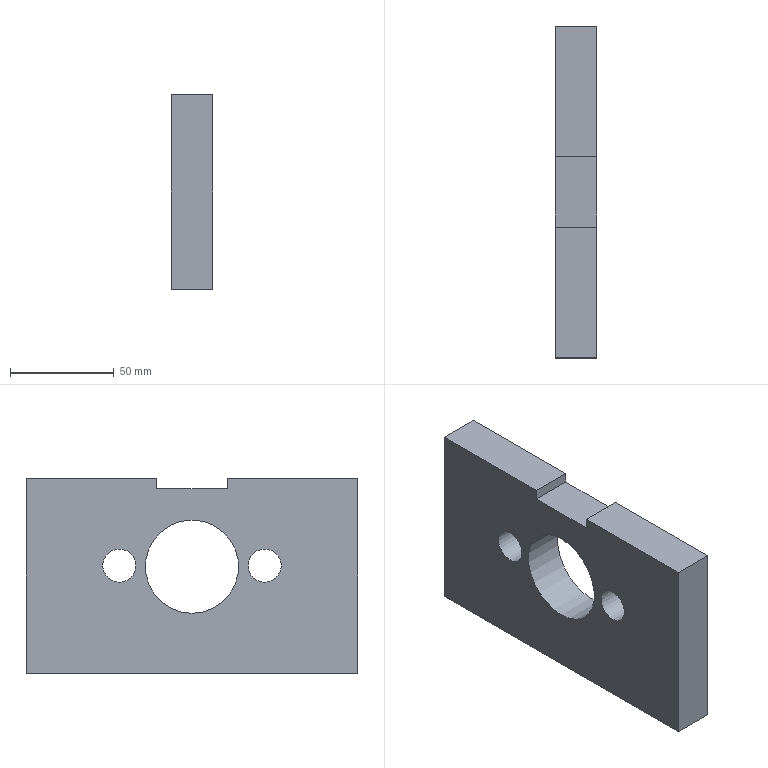Part | STEP file | Tube feed_id382_x_t | 1 solid | 13 faces | box 20 x 160 x 94 mm | volume 257549 mm3 | plane 10 | cylinder 3 | commonest cylinder face diameters 16 x2 45 x1
STEP:
#1=CARTESIAN_POINT('',(0.,0.,0.));
#2=DIRECTION('',(0.,0.,1.));
#3=DIRECTION('',(1.,0.,0.));
#4=AXIS2_PLACEMENT_3D('',#1,#2,#3);
#5=CARTESIAN_POINT('',(466.,446.936,-51.));
#6=VERTEX_POINT('',#5);
#7=CARTESIAN_POINT('',(466.,446.936,-43.));
#8=DIRECTION('',(-1.,0.,0.));
#9=DIRECTION('',(0.,0.,-1.));
#10=AXIS2_PLACEMENT_3D('',#7,#8,#9);
#11=CIRCLE('',#10,8.);
#12=CARTESIAN_POINT('',(466.,0.,0.));
#13=DIRECTION('',(1.,0.,0.));
#14=DIRECTION('',(0.,0.,-1.));
#15=AXIS2_PLACEMENT_3D('',#12,#13,#14);
#16=PLANE('',#15);
#17=CARTESIAN_POINT('',(51.,446.936));
#18=CARTESIAN_POINT('',(51.,433.079));
#19=CARTESIAN_POINT('',(39.,440.007));
#20=CARTESIAN_POINT('',(27.,446.936));
#21=CARTESIAN_POINT('',(39.,453.864));
#22=CARTESIAN_POINT('',(51.,460.792));
#23=CARTESIAN_POINT('',(51.,446.936));
#24=(BOUNDED_CURVE()B_SPLINE_CURVE(2,(#17,#18,#19,#20,#21,#22,#23),.UNSPECIFIED.,.T.,.F.)B_SPLINE_CURVE_WITH_KNOTS((1,2,2,2,2,1),(-2.094,0.,2.094,4.189,6.283,8.378),.UNSPECIFIED.)CURVE()GEOMETRIC_REPRESENTATION_ITEM()RATIONAL_B_SPLINE_CURVE((1.,0.5,1.,0.5,1.,0.5,1.))REPRESENTATION_ITEM(''));
#25=(GEOMETRIC_REPRESENTATION_CONTEXT(2)PARAMETRIC_REPRESENTATION_CONTEXT()REPRESENTATION_CONTEXT('',''));
#26=DEFINITIONAL_REPRESENTATION('',(#24),#25);
#27=PCURVE('',#16,#26);
#28=CARTESIAN_POINT('',(466.,446.936,-43.));
#29=DIRECTION('',(-1.,0.,0.));
#30=DIRECTION('',(0.,0.,1.));
#31=AXIS2_PLACEMENT_3D('',#28,#29,#30);
#32=CYLINDRICAL_SURFACE('',#31,8.);
#33=CARTESIAN_POINT('',(3.142,0.));
#34=DIRECTION('',(1.,0.));
#35=VECTOR('',#34,1.);
#36=LINE('',#33,#35);
#37=(GEOMETRIC_REPRESENTATION_CONTEXT(2)PARAMETRIC_REPRESENTATION_CONTEXT()REPRESENTATION_CONTEXT('',''));
#38=DEFINITIONAL_REPRESENTATION('',(#36),#37);
#39=PCURVE('',#32,#38);
#40=SURFACE_CURVE('',#11,(#27,#39),.PCURVE_S1.);
#41=EDGE_CURVE('',#6,#6,#40,.T.);
#42=ORIENTED_EDGE('',*,*,#41,.T.);
#43=EDGE_LOOP('',(#42));
#44=FACE_BOUND('',#43,.T.);
#45=CARTESIAN_POINT('',(466.,411.936,-66.));
#46=VERTEX_POINT('',#45);
#47=CARTESIAN_POINT('',(466.,411.936,-43.5));
#48=DIRECTION('',(-1.,0.,0.));
#49=DIRECTION('',(0.,0.,-1.));
#50=AXIS2_PLACEMENT_3D('',#47,#48,#49);
#51=CIRCLE('',#50,22.5);
#52=CARTESIAN_POINT('',(66.,411.936));
#53=CARTESIAN_POINT('',(66.,372.964));
#54=CARTESIAN_POINT('',(32.25,392.45));
#55=CARTESIAN_POINT('',(-1.5,411.936));
#56=CARTESIAN_POINT('',(32.25,431.421));
#57=CARTESIAN_POINT('',(66.,450.907));
#58=CARTESIAN_POINT('',(66.,411.936));
#59=(BOUNDED_CURVE()B_SPLINE_CURVE(2,(#52,#53,#54,#55,#56,#57,#58),.UNSPECIFIED.,.T.,.F.)B_SPLINE_CURVE_WITH_KNOTS((1,2,2,2,2,1),(-2.094,0.,2.094,4.189,6.283,8.378),.UNSPECIFIED.)CURVE()GEOMETRIC_REPRESENTATION_ITEM()RATIONAL_B_SPLINE_CURVE((1.,0.5,1.,0.5,1.,0.5,1.))REPRESENTATION_ITEM(''));
#60=(GEOMETRIC_REPRESENTATION_CONTEXT(2)PARAMETRIC_REPRESENTATION_CONTEXT()REPRESENTATION_CONTEXT('',''));
#61=DEFINITIONAL_REPRESENTATION('',(#59),#60);
#62=PCURVE('',#16,#61);
#63=CARTESIAN_POINT('',(398.5,411.936,-43.5));
#64=DIRECTION('',(1.,0.,0.));
#65=DIRECTION('',(0.,0.,-1.));
#66=AXIS2_PLACEMENT_3D('',#63,#64,#65);
#67=CYLINDRICAL_SURFACE('',#66,22.5);
#68=CARTESIAN_POINT('',(6.283,67.5));
#69=DIRECTION('',(-1.,0.));
#70=VECTOR('',#69,1.);
#71=LINE('',#68,#70);
#72=(GEOMETRIC_REPRESENTATION_CONTEXT(2)PARAMETRIC_REPRESENTATION_CONTEXT()REPRESENTATION_CONTEXT('',''));
#73=DEFINITIONAL_REPRESENTATION('',(#71),#72);
#74=PCURVE('',#67,#73);
#75=SURFACE_CURVE('',#51,(#62,#74),.PCURVE_S1.);
#76=EDGE_CURVE('',#46,#46,#75,.T.);
#77=ORIENTED_EDGE('',*,*,#76,.T.);
#78=EDGE_LOOP('',(#77));
#79=FACE_BOUND('',#78,.T.);
#80=CARTESIAN_POINT('',(466.,428.936,-6.));
#81=VERTEX_POINT('',#80);
#82=CARTESIAN_POINT('',(466.,394.936,-6.));
#83=VERTEX_POINT('',#82);
#84=CARTESIAN_POINT('',(466.,30.286,-6.));
#85=DIRECTION('',(0.,-1.,0.));
#86=VECTOR('',#85,1.);
#87=LINE('',#84,#86);
#88=CARTESIAN_POINT('',(6.,30.286));
#89=DIRECTION('',(0.,-1.));
#90=VECTOR('',#89,1.);
#91=LINE('',#88,#90);
#92=(GEOMETRIC_REPRESENTATION_CONTEXT(2)PARAMETRIC_REPRESENTATION_CONTEXT()REPRESENTATION_CONTEXT('',''));
#93=DEFINITIONAL_REPRESENTATION('',(#91),#92);
#94=PCURVE('',#16,#93);
#95=CARTESIAN_POINT('',(-249.,30.286,-6.));
#96=DIRECTION('',(0.,0.,1.));
#97=DIRECTION('',(0.,-1.,0.));
#98=AXIS2_PLACEMENT_3D('',#95,#96,#97);
#99=PLANE('',#98);
#100=CARTESIAN_POINT('',(0.,715.));
#101=DIRECTION('',(1.,0.));
#102=VECTOR('',#101,1.);
#103=LINE('',#100,#102);
#104=(GEOMETRIC_REPRESENTATION_CONTEXT(2)PARAMETRIC_REPRESENTATION_CONTEXT()REPRESENTATION_CONTEXT('',''));
#105=DEFINITIONAL_REPRESENTATION('',(#103),#104);
#106=PCURVE('',#99,#105);
#107=SURFACE_CURVE('',#87,(#94,#106),.PCURVE_S1.);
#108=EDGE_CURVE('',#81,#83,#107,.T.);
#109=ORIENTED_EDGE('',*,*,#108,.T.);
#110=CARTESIAN_POINT('',(466.,394.936,-1.));
#111=VERTEX_POINT('',#110);
#112=CARTESIAN_POINT('',(466.,394.936,0.));
#113=DIRECTION('',(0.,0.,-1.));
#114=VECTOR('',#113,1.);
#115=LINE('',#112,#114);
#116=CARTESIAN_POINT('',(0.,394.936));
#117=DIRECTION('',(1.,0.));
#118=VECTOR('',#117,1.);
#119=LINE('',#116,#118);
#120=(GEOMETRIC_REPRESENTATION_CONTEXT(2)PARAMETRIC_REPRESENTATION_CONTEXT()REPRESENTATION_CONTEXT('',''));
#121=DEFINITIONAL_REPRESENTATION('',(#119),#120);
#122=PCURVE('',#16,#121);
#123=CARTESIAN_POINT('',(21.,394.936,140.));
#124=DIRECTION('',(0.,-1.,0.));
#125=DIRECTION('',(0.,0.,-1.));
#126=AXIS2_PLACEMENT_3D('',#123,#124,#125);
#127=PLANE('',#126);
#128=CARTESIAN_POINT('',(140.,445.));
#129=DIRECTION('',(1.,0.));
#130=VECTOR('',#129,1.);
#131=LINE('',#128,#130);
#132=(GEOMETRIC_REPRESENTATION_CONTEXT(2)PARAMETRIC_REPRESENTATION_CONTEXT()REPRESENTATION_CONTEXT('',''));
#133=DEFINITIONAL_REPRESENTATION('',(#131),#132);
#134=PCURVE('',#127,#133);
#135=SURFACE_CURVE('',#115,(#122,#134),.PCURVE_S1.);
#136=EDGE_CURVE('',#111,#83,#135,.T.);
#137=ORIENTED_EDGE('',*,*,#136,.F.);
#138=CARTESIAN_POINT('',(466.,331.936,-1.));
#139=VERTEX_POINT('',#138);
#140=CARTESIAN_POINT('',(466.,0.,-1.));
#141=DIRECTION('',(0.,-1.,0.));
#142=VECTOR('',#141,1.);
#143=LINE('',#140,#142);
#144=CARTESIAN_POINT('',(1.,0.));
#145=DIRECTION('',(0.,-1.));
#146=VECTOR('',#145,1.);
#147=LINE('',#144,#146);
#148=(GEOMETRIC_REPRESENTATION_CONTEXT(2)PARAMETRIC_REPRESENTATION_CONTEXT()REPRESENTATION_CONTEXT('',''));
#149=DEFINITIONAL_REPRESENTATION('',(#147),#148);
#150=PCURVE('',#16,#149);
#151=CARTESIAN_POINT('',(-249.,30.286,-1.));
#152=DIRECTION('',(0.,0.,1.));
#153=DIRECTION('',(0.,-1.,0.));
#154=AXIS2_PLACEMENT_3D('',#151,#152,#153);
#155=PLANE('',#154);
#156=CARTESIAN_POINT('',(30.286,715.));
#157=DIRECTION('',(1.,0.));
#158=VECTOR('',#157,1.);
#159=LINE('',#156,#158);
#160=(GEOMETRIC_REPRESENTATION_CONTEXT(2)PARAMETRIC_REPRESENTATION_CONTEXT()REPRESENTATION_CONTEXT('',''));
#161=DEFINITIONAL_REPRESENTATION('',(#159),#160);
#162=PCURVE('',#155,#161);
#163=SURFACE_CURVE('',#143,(#150,#162),.PCURVE_S1.);
#164=EDGE_CURVE('',#111,#139,#163,.T.);
#165=ORIENTED_EDGE('',*,*,#164,.T.);
#166=CARTESIAN_POINT('',(466.,331.936,-95.));
#167=VERTEX_POINT('',#166);
#168=CARTESIAN_POINT('',(466.,331.936,5.));
#169=DIRECTION('',(0.,0.,-1.));
#170=VECTOR('',#169,1.);
#171=LINE('',#168,#170);
#172=CARTESIAN_POINT('',(-5.,331.936));
#173=DIRECTION('',(1.,0.));
#174=VECTOR('',#173,1.);
#175=LINE('',#172,#174);
#176=(GEOMETRIC_REPRESENTATION_CONTEXT(2)PARAMETRIC_REPRESENTATION_CONTEXT()REPRESENTATION_CONTEXT('',''));
#177=DEFINITIONAL_REPRESENTATION('',(#175),#176);
#178=PCURVE('',#16,#177);
#179=CARTESIAN_POINT('',(446.,331.936,5.));
#180=DIRECTION('',(0.,-1.,0.));
#181=DIRECTION('',(0.,0.,-1.));
#182=AXIS2_PLACEMENT_3D('',#179,#180,#181);
#183=PLANE('',#182);
#184=CARTESIAN_POINT('',(0.,20.));
#185=DIRECTION('',(1.,0.));
#186=VECTOR('',#185,1.);
#187=LINE('',#184,#186);
#188=(GEOMETRIC_REPRESENTATION_CONTEXT(2)PARAMETRIC_REPRESENTATION_CONTEXT()REPRESENTATION_CONTEXT('',''));
#189=DEFINITIONAL_REPRESENTATION('',(#187),#188);
#190=PCURVE('',#183,#189);
#191=SURFACE_CURVE('',#171,(#178,#190),.PCURVE_S1.);
#192=EDGE_CURVE('',#139,#167,#191,.T.);
#193=ORIENTED_EDGE('',*,*,#192,.T.);
#194=CARTESIAN_POINT('',(466.,491.936,-95.));
#195=VERTEX_POINT('',#194);
#196=CARTESIAN_POINT('',(466.,331.936,-95.));
#197=DIRECTION('',(0.,1.,0.));
#198=VECTOR('',#197,1.);
#199=LINE('',#196,#198);
#200=CARTESIAN_POINT('',(95.,331.936));
#201=DIRECTION('',(0.,1.));
#202=VECTOR('',#201,1.);
#203=LINE('',#200,#202);
#204=(GEOMETRIC_REPRESENTATION_CONTEXT(2)PARAMETRIC_REPRESENTATION_CONTEXT()REPRESENTATION_CONTEXT('',''));
#205=DEFINITIONAL_REPRESENTATION('',(#203),#204);
#206=PCURVE('',#16,#205);
#207=CARTESIAN_POINT('',(446.,331.936,-95.));
#208=DIRECTION('',(0.,0.,-1.));
#209=DIRECTION('',(0.,1.,0.));
#210=AXIS2_PLACEMENT_3D('',#207,#208,#209);
#211=PLANE('',#210);
#212=CARTESIAN_POINT('',(0.,20.));
#213=DIRECTION('',(1.,0.));
#214=VECTOR('',#213,1.);
#215=LINE('',#212,#214);
#216=(GEOMETRIC_REPRESENTATION_CONTEXT(2)PARAMETRIC_REPRESENTATION_CONTEXT()REPRESENTATION_CONTEXT('',''));
#217=DEFINITIONAL_REPRESENTATION('',(#215),#216);
#218=PCURVE('',#211,#217);
#219=SURFACE_CURVE('',#199,(#206,#218),.PCURVE_S1.);
#220=EDGE_CURVE('',#167,#195,#219,.T.);
#221=ORIENTED_EDGE('',*,*,#220,.T.);
#222=CARTESIAN_POINT('',(466.,491.936,-1.));
#223=VERTEX_POINT('',#222);
#224=CARTESIAN_POINT('',(466.,491.936,-95.));
#225=DIRECTION('',(0.,0.,1.));
#226=VECTOR('',#225,1.);
#227=LINE('',#224,#226);
#228=CARTESIAN_POINT('',(95.,491.936));
#229=DIRECTION('',(-1.,0.));
#230=VECTOR('',#229,1.);
#231=LINE('',#228,#230);
#232=(GEOMETRIC_REPRESENTATION_CONTEXT(2)PARAMETRIC_REPRESENTATION_CONTEXT()REPRESENTATION_CONTEXT('',''));
#233=DEFINITIONAL_REPRESENTATION('',(#231),#232);
#234=PCURVE('',#16,#233);
#235=CARTESIAN_POINT('',(446.,491.936,-95.));
#236=DIRECTION('',(0.,1.,0.));
#237=DIRECTION('',(0.,0.,1.));
#238=AXIS2_PLACEMENT_3D('',#235,#236,#237);
#239=PLANE('',#238);
#240=CARTESIAN_POINT('',(0.,20.));
#241=DIRECTION('',(1.,0.));
#242=VECTOR('',#241,1.);
#243=LINE('',#240,#242);
#244=(GEOMETRIC_REPRESENTATION_CONTEXT(2)PARAMETRIC_REPRESENTATION_CONTEXT()REPRESENTATION_CONTEXT('',''));
#245=DEFINITIONAL_REPRESENTATION('',(#243),#244);
#246=PCURVE('',#239,#245);
#247=SURFACE_CURVE('',#227,(#234,#246),.PCURVE_S1.);
#248=EDGE_CURVE('',#195,#223,#247,.T.);
#249=ORIENTED_EDGE('',*,*,#248,.T.);
#250=CARTESIAN_POINT('',(466.,428.936,-1.));
#251=VERTEX_POINT('',#250);
#252=CARTESIAN_POINT('',(466.,0.,-1.));
#253=DIRECTION('',(0.,-1.,0.));
#254=VECTOR('',#253,1.);
#255=LINE('',#252,#254);
#256=CARTESIAN_POINT('',(1.,0.));
#257=DIRECTION('',(0.,-1.));
#258=VECTOR('',#257,1.);
#259=LINE('',#256,#258);
#260=(GEOMETRIC_REPRESENTATION_CONTEXT(2)PARAMETRIC_REPRESENTATION_CONTEXT()REPRESENTATION_CONTEXT('',''));
#261=DEFINITIONAL_REPRESENTATION('',(#259),#260);
#262=PCURVE('',#16,#261);
#263=CARTESIAN_POINT('',(-249.,30.286,-1.));
#264=DIRECTION('',(0.,0.,1.));
#265=DIRECTION('',(0.,-1.,0.));
#266=AXIS2_PLACEMENT_3D('',#263,#264,#265);
#267=PLANE('',#266);
#268=CARTESIAN_POINT('',(30.286,715.));
#269=DIRECTION('',(1.,0.));
#270=VECTOR('',#269,1.);
#271=LINE('',#268,#270);
#272=(GEOMETRIC_REPRESENTATION_CONTEXT(2)PARAMETRIC_REPRESENTATION_CONTEXT()REPRESENTATION_CONTEXT('',''));
#273=DEFINITIONAL_REPRESENTATION('',(#271),#272);
#274=PCURVE('',#267,#273);
#275=SURFACE_CURVE('',#255,(#262,#274),.PCURVE_S1.);
#276=EDGE_CURVE('',#223,#251,#275,.T.);
#277=ORIENTED_EDGE('',*,*,#276,.T.);
#278=CARTESIAN_POINT('',(466.,428.936,140.));
#279=DIRECTION('',(0.,0.,-1.));
#280=VECTOR('',#279,1.);
#281=LINE('',#278,#280);
#282=CARTESIAN_POINT('',(-140.,428.936));
#283=DIRECTION('',(1.,0.));
#284=VECTOR('',#283,1.);
#285=LINE('',#282,#284);
#286=(GEOMETRIC_REPRESENTATION_CONTEXT(2)PARAMETRIC_REPRESENTATION_CONTEXT()REPRESENTATION_CONTEXT('',''));
#287=DEFINITIONAL_REPRESENTATION('',(#285),#286);
#288=PCURVE('',#16,#287);
#289=CARTESIAN_POINT('',(-4.,428.936,140.));
#290=DIRECTION('',(0.,1.,0.));
#291=DIRECTION('',(-1.,0.,0.));
#292=AXIS2_PLACEMENT_3D('',#289,#290,#291);
#293=PLANE('',#292);
#294=CARTESIAN_POINT('',(-470.,0.));
#295=DIRECTION('',(0.,-1.));
#296=VECTOR('',#295,1.);
#297=LINE('',#294,#296);
#298=(GEOMETRIC_REPRESENTATION_CONTEXT(2)PARAMETRIC_REPRESENTATION_CONTEXT()REPRESENTATION_CONTEXT('',''));
#299=DEFINITIONAL_REPRESENTATION('',(#297),#298);
#300=PCURVE('',#293,#299);
#301=SURFACE_CURVE('',#281,(#288,#300),.PCURVE_S1.);
#302=EDGE_CURVE('',#251,#81,#301,.T.);
#303=ORIENTED_EDGE('',*,*,#302,.T.);
#304=EDGE_LOOP('',(#109,#137,#165,#193,#221,#249,#277,#303));
#305=FACE_BOUND('',#304,.T.);
#306=CARTESIAN_POINT('',(466.,376.936,-51.));
#307=VERTEX_POINT('',#306);
#308=CARTESIAN_POINT('',(466.,376.936,-43.));
#309=DIRECTION('',(-1.,0.,0.));
#310=DIRECTION('',(0.,0.,-1.));
#311=AXIS2_PLACEMENT_3D('',#308,#309,#310);
#312=CIRCLE('',#311,8.);
#313=CARTESIAN_POINT('',(51.,376.936));
#314=CARTESIAN_POINT('',(51.,363.079));
#315=CARTESIAN_POINT('',(39.,370.007));
#316=CARTESIAN_POINT('',(27.,376.936));
#317=CARTESIAN_POINT('',(39.,383.864));
#318=CARTESIAN_POINT('',(51.,390.792));
#319=CARTESIAN_POINT('',(51.,376.936));
#320=(BOUNDED_CURVE()B_SPLINE_CURVE(2,(#313,#314,#315,#316,#317,#318,#319),.UNSPECIFIED.,.T.,.F.)B_SPLINE_CURVE_WITH_KNOTS((1,2,2,2,2,1),(-2.094,0.,2.094,4.189,6.283,8.378),.UNSPECIFIED.)CURVE()GEOMETRIC_REPRESENTATION_ITEM()RATIONAL_B_SPLINE_CURVE((1.,0.5,1.,0.5,1.,0.5,1.))REPRESENTATION_ITEM(''));
#321=(GEOMETRIC_REPRESENTATION_CONTEXT(2)PARAMETRIC_REPRESENTATION_CONTEXT()REPRESENTATION_CONTEXT('',''));
#322=DEFINITIONAL_REPRESENTATION('',(#320),#321);
#323=PCURVE('',#16,#322);
#324=CARTESIAN_POINT('',(466.,376.936,-43.));
#325=DIRECTION('',(-1.,0.,0.));
#326=DIRECTION('',(0.,0.,1.));
#327=AXIS2_PLACEMENT_3D('',#324,#325,#326);
#328=CYLINDRICAL_SURFACE('',#327,8.);
#329=CARTESIAN_POINT('',(3.142,0.));
#330=DIRECTION('',(1.,0.));
#331=VECTOR('',#330,1.);
#332=LINE('',#329,#331);
#333=(GEOMETRIC_REPRESENTATION_CONTEXT(2)PARAMETRIC_REPRESENTATION_CONTEXT()REPRESENTATION_CONTEXT('',''));
#334=DEFINITIONAL_REPRESENTATION('',(#332),#333);
#335=PCURVE('',#328,#334);
#336=SURFACE_CURVE('',#312,(#323,#335),.PCURVE_S1.);
#337=EDGE_CURVE('',#307,#307,#336,.T.);
#338=ORIENTED_EDGE('',*,*,#337,.T.);
#339=EDGE_LOOP('',(#338));
#340=FACE_BOUND('',#339,.T.);
#341=ADVANCED_FACE('',(#44,#79,#305,#340),#16,.T.);
#342=CARTESIAN_POINT('',(446.,428.936,-1.));
#343=VERTEX_POINT('',#342);
#344=CARTESIAN_POINT('',(446.,428.936,-6.));
#345=VERTEX_POINT('',#344);
#346=CARTESIAN_POINT('',(446.,428.936,140.));
#347=DIRECTION('',(0.,0.,-1.));
#348=VECTOR('',#347,1.);
#349=LINE('',#346,#348);
#350=CARTESIAN_POINT('',(446.,0.,0.));
#351=DIRECTION('',(1.,0.,0.));
#352=DIRECTION('',(0.,0.,-1.));
#353=AXIS2_PLACEMENT_3D('',#350,#351,#352);
#354=PLANE('',#353);
#355=CARTESIAN_POINT('',(-140.,428.936));
#356=DIRECTION('',(1.,0.));
#357=VECTOR('',#356,1.);
#358=LINE('',#355,#357);
#359=(GEOMETRIC_REPRESENTATION_CONTEXT(2)PARAMETRIC_REPRESENTATION_CONTEXT()REPRESENTATION_CONTEXT('',''));
#360=DEFINITIONAL_REPRESENTATION('',(#358),#359);
#361=PCURVE('',#354,#360);
#362=CARTESIAN_POINT('',(-450.,0.));
#363=DIRECTION('',(0.,-1.));
#364=VECTOR('',#363,1.);
#365=LINE('',#362,#364);
#366=(GEOMETRIC_REPRESENTATION_CONTEXT(2)PARAMETRIC_REPRESENTATION_CONTEXT()REPRESENTATION_CONTEXT('',''));
#367=DEFINITIONAL_REPRESENTATION('',(#365),#366);
#368=PCURVE('',#293,#367);
#369=SURFACE_CURVE('',#349,(#361,#368),.PCURVE_S1.);
#370=EDGE_CURVE('',#343,#345,#369,.T.);
#371=ORIENTED_EDGE('',*,*,#370,.F.);
#372=CARTESIAN_POINT('',(446.,491.936,-1.));
#373=VERTEX_POINT('',#372);
#374=CARTESIAN_POINT('',(446.,0.,-1.));
#375=DIRECTION('',(0.,-1.,0.));
#376=VECTOR('',#375,1.);
#377=LINE('',#374,#376);
#378=CARTESIAN_POINT('',(1.,0.));
#379=DIRECTION('',(0.,-1.));
#380=VECTOR('',#379,1.);
#381=LINE('',#378,#380);
#382=(GEOMETRIC_REPRESENTATION_CONTEXT(2)PARAMETRIC_REPRESENTATION_CONTEXT()REPRESENTATION_CONTEXT('',''));
#383=DEFINITIONAL_REPRESENTATION('',(#381),#382);
#384=PCURVE('',#354,#383);
#385=CARTESIAN_POINT('',(30.286,695.));
#386=DIRECTION('',(1.,0.));
#387=VECTOR('',#386,1.);
#388=LINE('',#385,#387);
#389=(GEOMETRIC_REPRESENTATION_CONTEXT(2)PARAMETRIC_REPRESENTATION_CONTEXT()REPRESENTATION_CONTEXT('',''));
#390=DEFINITIONAL_REPRESENTATION('',(#388),#389);
#391=PCURVE('',#267,#390);
#392=SURFACE_CURVE('',#377,(#384,#391),.PCURVE_S1.);
#393=EDGE_CURVE('',#373,#343,#392,.T.);
#394=ORIENTED_EDGE('',*,*,#393,.F.);
#395=CARTESIAN_POINT('',(446.,491.936,-95.));
#396=VERTEX_POINT('',#395);
#397=CARTESIAN_POINT('',(446.,491.936,-95.));
#398=DIRECTION('',(0.,0.,1.));
#399=VECTOR('',#398,1.);
#400=LINE('',#397,#399);
#401=CARTESIAN_POINT('',(95.,491.936));
#402=DIRECTION('',(-1.,0.));
#403=VECTOR('',#402,1.);
#404=LINE('',#401,#403);
#405=(GEOMETRIC_REPRESENTATION_CONTEXT(2)PARAMETRIC_REPRESENTATION_CONTEXT()REPRESENTATION_CONTEXT('',''));
#406=DEFINITIONAL_REPRESENTATION('',(#404),#405);
#407=PCURVE('',#354,#406);
#408=CARTESIAN_POINT('',(0.,0.));
#409=DIRECTION('',(1.,0.));
#410=VECTOR('',#409,1.);
#411=LINE('',#408,#410);
#412=(GEOMETRIC_REPRESENTATION_CONTEXT(2)PARAMETRIC_REPRESENTATION_CONTEXT()REPRESENTATION_CONTEXT('',''));
#413=DEFINITIONAL_REPRESENTATION('',(#411),#412);
#414=PCURVE('',#239,#413);
#415=SURFACE_CURVE('',#400,(#407,#414),.PCURVE_S1.);
#416=EDGE_CURVE('',#396,#373,#415,.T.);
#417=ORIENTED_EDGE('',*,*,#416,.F.);
#418=CARTESIAN_POINT('',(446.,331.936,-95.));
#419=VERTEX_POINT('',#418);
#420=CARTESIAN_POINT('',(446.,331.936,-95.));
#421=DIRECTION('',(0.,1.,0.));
#422=VECTOR('',#421,1.);
#423=LINE('',#420,#422);
#424=CARTESIAN_POINT('',(95.,331.936));
#425=DIRECTION('',(0.,1.));
#426=VECTOR('',#425,1.);
#427=LINE('',#424,#426);
#428=(GEOMETRIC_REPRESENTATION_CONTEXT(2)PARAMETRIC_REPRESENTATION_CONTEXT()REPRESENTATION_CONTEXT('',''));
#429=DEFINITIONAL_REPRESENTATION('',(#427),#428);
#430=PCURVE('',#354,#429);
#431=CARTESIAN_POINT('',(0.,0.));
#432=DIRECTION('',(1.,0.));
#433=VECTOR('',#432,1.);
#434=LINE('',#431,#433);
#435=(GEOMETRIC_REPRESENTATION_CONTEXT(2)PARAMETRIC_REPRESENTATION_CONTEXT()REPRESENTATION_CONTEXT('',''));
#436=DEFINITIONAL_REPRESENTATION('',(#434),#435);
#437=PCURVE('',#211,#436);
#438=SURFACE_CURVE('',#423,(#430,#437),.PCURVE_S1.);
#439=EDGE_CURVE('',#419,#396,#438,.T.);
#440=ORIENTED_EDGE('',*,*,#439,.F.);
#441=CARTESIAN_POINT('',(446.,331.936,-1.));
#442=VERTEX_POINT('',#441);
#443=CARTESIAN_POINT('',(446.,331.936,5.));
#444=DIRECTION('',(0.,0.,-1.));
#445=VECTOR('',#444,1.);
#446=LINE('',#443,#445);
#447=CARTESIAN_POINT('',(-5.,331.936));
#448=DIRECTION('',(1.,0.));
#449=VECTOR('',#448,1.);
#450=LINE('',#447,#449);
#451=(GEOMETRIC_REPRESENTATION_CONTEXT(2)PARAMETRIC_REPRESENTATION_CONTEXT()REPRESENTATION_CONTEXT('',''));
#452=DEFINITIONAL_REPRESENTATION('',(#450),#451);
#453=PCURVE('',#354,#452);
#454=CARTESIAN_POINT('',(0.,0.));
#455=DIRECTION('',(1.,0.));
#456=VECTOR('',#455,1.);
#457=LINE('',#454,#456);
#458=(GEOMETRIC_REPRESENTATION_CONTEXT(2)PARAMETRIC_REPRESENTATION_CONTEXT()REPRESENTATION_CONTEXT('',''));
#459=DEFINITIONAL_REPRESENTATION('',(#457),#458);
#460=PCURVE('',#183,#459);
#461=SURFACE_CURVE('',#446,(#453,#460),.PCURVE_S1.);
#462=EDGE_CURVE('',#442,#419,#461,.T.);
#463=ORIENTED_EDGE('',*,*,#462,.F.);
#464=CARTESIAN_POINT('',(446.,394.936,-1.));
#465=VERTEX_POINT('',#464);
#466=CARTESIAN_POINT('',(446.,0.,-1.));
#467=DIRECTION('',(0.,-1.,0.));
#468=VECTOR('',#467,1.);
#469=LINE('',#466,#468);
#470=CARTESIAN_POINT('',(1.,0.));
#471=DIRECTION('',(0.,-1.));
#472=VECTOR('',#471,1.);
#473=LINE('',#470,#472);
#474=(GEOMETRIC_REPRESENTATION_CONTEXT(2)PARAMETRIC_REPRESENTATION_CONTEXT()REPRESENTATION_CONTEXT('',''));
#475=DEFINITIONAL_REPRESENTATION('',(#473),#474);
#476=PCURVE('',#354,#475);
#477=CARTESIAN_POINT('',(30.286,695.));
#478=DIRECTION('',(1.,0.));
#479=VECTOR('',#478,1.);
#480=LINE('',#477,#479);
#481=(GEOMETRIC_REPRESENTATION_CONTEXT(2)PARAMETRIC_REPRESENTATION_CONTEXT()REPRESENTATION_CONTEXT('',''));
#482=DEFINITIONAL_REPRESENTATION('',(#480),#481);
#483=PCURVE('',#155,#482);
#484=SURFACE_CURVE('',#469,(#476,#483),.PCURVE_S1.);
#485=EDGE_CURVE('',#465,#442,#484,.T.);
#486=ORIENTED_EDGE('',*,*,#485,.F.);
#487=CARTESIAN_POINT('',(446.,394.936,-6.));
#488=VERTEX_POINT('',#487);
#489=CARTESIAN_POINT('',(446.,394.936,0.));
#490=DIRECTION('',(0.,0.,-1.));
#491=VECTOR('',#490,1.);
#492=LINE('',#489,#491);
#493=CARTESIAN_POINT('',(0.,394.936));
#494=DIRECTION('',(1.,0.));
#495=VECTOR('',#494,1.);
#496=LINE('',#493,#495);
#497=(GEOMETRIC_REPRESENTATION_CONTEXT(2)PARAMETRIC_REPRESENTATION_CONTEXT()REPRESENTATION_CONTEXT('',''));
#498=DEFINITIONAL_REPRESENTATION('',(#496),#497);
#499=PCURVE('',#354,#498);
#500=CARTESIAN_POINT('',(140.,425.));
#501=DIRECTION('',(1.,0.));
#502=VECTOR('',#501,1.);
#503=LINE('',#500,#502);
#504=(GEOMETRIC_REPRESENTATION_CONTEXT(2)PARAMETRIC_REPRESENTATION_CONTEXT()REPRESENTATION_CONTEXT('',''));
#505=DEFINITIONAL_REPRESENTATION('',(#503),#504);
#506=PCURVE('',#127,#505);
#507=SURFACE_CURVE('',#492,(#499,#506),.PCURVE_S1.);
#508=EDGE_CURVE('',#465,#488,#507,.T.);
#509=ORIENTED_EDGE('',*,*,#508,.T.);
#510=CARTESIAN_POINT('',(446.,0.,-6.));
#511=DIRECTION('',(0.,1.,0.));
#512=VECTOR('',#511,1.);
#513=LINE('',#510,#512);
#514=CARTESIAN_POINT('',(6.,0.));
#515=DIRECTION('',(0.,1.));
#516=VECTOR('',#515,1.);
#517=LINE('',#514,#516);
#518=(GEOMETRIC_REPRESENTATION_CONTEXT(2)PARAMETRIC_REPRESENTATION_CONTEXT()REPRESENTATION_CONTEXT('',''));
#519=DEFINITIONAL_REPRESENTATION('',(#517),#518);
#520=PCURVE('',#354,#519);
#521=CARTESIAN_POINT('',(30.286,695.));
#522=DIRECTION('',(-1.,0.));
#523=VECTOR('',#522,1.);
#524=LINE('',#521,#523);
#525=(GEOMETRIC_REPRESENTATION_CONTEXT(2)PARAMETRIC_REPRESENTATION_CONTEXT()REPRESENTATION_CONTEXT('',''));
#526=DEFINITIONAL_REPRESENTATION('',(#524),#525);
#527=PCURVE('',#99,#526);
#528=SURFACE_CURVE('',#513,(#520,#527),.PCURVE_S1.);
#529=EDGE_CURVE('',#488,#345,#528,.T.);
#530=ORIENTED_EDGE('',*,*,#529,.T.);
#531=EDGE_LOOP('',(#371,#394,#417,#440,#463,#486,#509,#530));
#532=FACE_BOUND('',#531,.T.);
#533=CARTESIAN_POINT('',(446.,411.936,-66.));
#534=VERTEX_POINT('',#533);
#535=CARTESIAN_POINT('',(446.,411.936,-43.5));
#536=DIRECTION('',(-1.,0.,0.));
#537=DIRECTION('',(0.,0.,-1.));
#538=AXIS2_PLACEMENT_3D('',#535,#536,#537);
#539=CIRCLE('',#538,22.5);
#540=CARTESIAN_POINT('',(66.,411.936));
#541=CARTESIAN_POINT('',(66.,372.964));
#542=CARTESIAN_POINT('',(32.25,392.45));
#543=CARTESIAN_POINT('',(-1.5,411.936));
#544=CARTESIAN_POINT('',(32.25,431.421));
#545=CARTESIAN_POINT('',(66.,450.907));
#546=CARTESIAN_POINT('',(66.,411.936));
#547=(BOUNDED_CURVE()B_SPLINE_CURVE(2,(#540,#541,#542,#543,#544,#545,#546),.UNSPECIFIED.,.T.,.F.)B_SPLINE_CURVE_WITH_KNOTS((1,2,2,2,2,1),(-2.094,0.,2.094,4.189,6.283,8.378),.UNSPECIFIED.)CURVE()GEOMETRIC_REPRESENTATION_ITEM()RATIONAL_B_SPLINE_CURVE((1.,0.5,1.,0.5,1.,0.5,1.))REPRESENTATION_ITEM(''));
#548=(GEOMETRIC_REPRESENTATION_CONTEXT(2)PARAMETRIC_REPRESENTATION_CONTEXT()REPRESENTATION_CONTEXT('',''));
#549=DEFINITIONAL_REPRESENTATION('',(#547),#548);
#550=PCURVE('',#354,#549);
#551=CARTESIAN_POINT('',(6.283,47.5));
#552=DIRECTION('',(-1.,0.));
#553=VECTOR('',#552,1.);
#554=LINE('',#551,#553);
#555=(GEOMETRIC_REPRESENTATION_CONTEXT(2)PARAMETRIC_REPRESENTATION_CONTEXT()REPRESENTATION_CONTEXT('',''));
#556=DEFINITIONAL_REPRESENTATION('',(#554),#555);
#557=PCURVE('',#67,#556);
#558=SURFACE_CURVE('',#539,(#550,#557),.PCURVE_S1.);
#559=EDGE_CURVE('',#534,#534,#558,.T.);
#560=ORIENTED_EDGE('',*,*,#559,.F.);
#561=EDGE_LOOP('',(#560));
#562=FACE_BOUND('',#561,.T.);
#563=CARTESIAN_POINT('',(446.,376.936,-51.));
#564=VERTEX_POINT('',#563);
#565=CARTESIAN_POINT('',(446.,376.936,-43.));
#566=DIRECTION('',(1.,0.,0.));
#567=DIRECTION('',(0.,0.,-1.));
#568=AXIS2_PLACEMENT_3D('',#565,#566,#567);
#569=CIRCLE('',#568,8.);
#570=CARTESIAN_POINT('',(43.,376.936));
#571=DIRECTION('',(1.,0.));
#572=AXIS2_PLACEMENT_2D('',#570,#571);
#573=CIRCLE('',#572,8.);
#574=(GEOMETRIC_REPRESENTATION_CONTEXT(2)PARAMETRIC_REPRESENTATION_CONTEXT()REPRESENTATION_CONTEXT('',''));
#575=DEFINITIONAL_REPRESENTATION('',(#573),#574);
#576=PCURVE('',#354,#575);
#577=CARTESIAN_POINT('',(9.425,20.));
#578=DIRECTION('',(-1.,0.));
#579=VECTOR('',#578,1.);
#580=LINE('',#577,#579);
#581=(GEOMETRIC_REPRESENTATION_CONTEXT(2)PARAMETRIC_REPRESENTATION_CONTEXT()REPRESENTATION_CONTEXT('',''));
#582=DEFINITIONAL_REPRESENTATION('',(#580),#581);
#583=PCURVE('',#328,#582);
#584=SURFACE_CURVE('',#569,(#576,#583),.PCURVE_S1.);
#585=EDGE_CURVE('',#564,#564,#584,.T.);
#586=ORIENTED_EDGE('',*,*,#585,.T.);
#587=EDGE_LOOP('',(#586));
#588=FACE_BOUND('',#587,.T.);
#589=CARTESIAN_POINT('',(446.,446.936,-51.));
#590=VERTEX_POINT('',#589);
#591=CARTESIAN_POINT('',(446.,446.936,-43.));
#592=DIRECTION('',(1.,0.,0.));
#593=DIRECTION('',(0.,0.,-1.));
#594=AXIS2_PLACEMENT_3D('',#591,#592,#593);
#595=CIRCLE('',#594,8.);
#596=CARTESIAN_POINT('',(43.,446.936));
#597=DIRECTION('',(1.,0.));
#598=AXIS2_PLACEMENT_2D('',#596,#597);
#599=CIRCLE('',#598,8.);
#600=(GEOMETRIC_REPRESENTATION_CONTEXT(2)PARAMETRIC_REPRESENTATION_CONTEXT()REPRESENTATION_CONTEXT('',''));
#601=DEFINITIONAL_REPRESENTATION('',(#599),#600);
#602=PCURVE('',#354,#601);
#603=CARTESIAN_POINT('',(9.425,20.));
#604=DIRECTION('',(-1.,0.));
#605=VECTOR('',#604,1.);
#606=LINE('',#603,#605);
#607=(GEOMETRIC_REPRESENTATION_CONTEXT(2)PARAMETRIC_REPRESENTATION_CONTEXT()REPRESENTATION_CONTEXT('',''));
#608=DEFINITIONAL_REPRESENTATION('',(#606),#607);
#609=PCURVE('',#32,#608);
#610=SURFACE_CURVE('',#595,(#602,#609),.PCURVE_S1.);
#611=EDGE_CURVE('',#590,#590,#610,.T.);
#612=ORIENTED_EDGE('',*,*,#611,.T.);
#613=EDGE_LOOP('',(#612));
#614=FACE_BOUND('',#613,.T.);
#615=ADVANCED_FACE('',(#532,#562,#588,#614),#354,.F.);
#616=CARTESIAN_POINT('',(-249.,428.936,-1.));
#617=DIRECTION('',(-1.,0.,0.));
#618=VECTOR('',#617,1.);
#619=LINE('',#616,#618);
#620=CARTESIAN_POINT('',(-398.65,0.));
#621=DIRECTION('',(0.,-1.));
#622=VECTOR('',#621,1.);
#623=LINE('',#620,#622);
#624=(GEOMETRIC_REPRESENTATION_CONTEXT(2)PARAMETRIC_REPRESENTATION_CONTEXT()REPRESENTATION_CONTEXT('',''));
#625=DEFINITIONAL_REPRESENTATION('',(#623),#624);
#626=PCURVE('',#267,#625);
#627=CARTESIAN_POINT('',(245.,-141.));
#628=DIRECTION('',(1.,0.));
#629=VECTOR('',#628,1.);
#630=LINE('',#627,#629);
#631=(GEOMETRIC_REPRESENTATION_CONTEXT(2)PARAMETRIC_REPRESENTATION_CONTEXT()REPRESENTATION_CONTEXT('',''));
#632=DEFINITIONAL_REPRESENTATION('',(#630),#631);
#633=PCURVE('',#293,#632);
#634=SURFACE_CURVE('',#619,(#626,#633),.PCURVE_S1.);
#635=EDGE_CURVE('',#251,#343,#634,.T.);
#636=ORIENTED_EDGE('',*,*,#635,.F.);
#637=ORIENTED_EDGE('',*,*,#276,.F.);
#638=CARTESIAN_POINT('',(446.,491.936,-1.));
#639=DIRECTION('',(1.,0.,0.));
#640=VECTOR('',#639,1.);
#641=LINE('',#638,#640);
#642=CARTESIAN_POINT('',(-461.65,695.));
#643=DIRECTION('',(0.,1.));
#644=VECTOR('',#643,1.);
#645=LINE('',#642,#644);
#646=(GEOMETRIC_REPRESENTATION_CONTEXT(2)PARAMETRIC_REPRESENTATION_CONTEXT()REPRESENTATION_CONTEXT('',''));
#647=DEFINITIONAL_REPRESENTATION('',(#645),#646);
#648=PCURVE('',#267,#647);
#649=CARTESIAN_POINT('',(94.,0.));
#650=DIRECTION('',(0.,1.));
#651=VECTOR('',#650,1.);
#652=LINE('',#649,#651);
#653=(GEOMETRIC_REPRESENTATION_CONTEXT(2)PARAMETRIC_REPRESENTATION_CONTEXT()REPRESENTATION_CONTEXT('',''));
#654=DEFINITIONAL_REPRESENTATION('',(#652),#653);
#655=PCURVE('',#239,#654);
#656=SURFACE_CURVE('',#641,(#648,#655),.PCURVE_S1.);
#657=EDGE_CURVE('',#373,#223,#656,.T.);
#658=ORIENTED_EDGE('',*,*,#657,.F.);
#659=ORIENTED_EDGE('',*,*,#393,.T.);
#660=EDGE_LOOP('',(#636,#637,#658,#659));
#661=FACE_BOUND('',#660,.T.);
#662=ADVANCED_FACE('',(#661),#267,.T.);
#663=ORIENTED_EDGE('',*,*,#192,.F.);
#664=CARTESIAN_POINT('',(-249.,331.936,-1.));
#665=DIRECTION('',(1.,0.,0.));
#666=VECTOR('',#665,1.);
#667=LINE('',#664,#666);
#668=CARTESIAN_POINT('',(6.,-695.));
#669=DIRECTION('',(0.,1.));
#670=VECTOR('',#669,1.);
#671=LINE('',#668,#670);
#672=(GEOMETRIC_REPRESENTATION_CONTEXT(2)PARAMETRIC_REPRESENTATION_CONTEXT()REPRESENTATION_CONTEXT('',''));
#673=DEFINITIONAL_REPRESENTATION('',(#671),#672);
#674=PCURVE('',#183,#673);
#675=CARTESIAN_POINT('',(-301.65,0.));
#676=DIRECTION('',(0.,1.));
#677=VECTOR('',#676,1.);
#678=LINE('',#675,#677);
#679=(GEOMETRIC_REPRESENTATION_CONTEXT(2)PARAMETRIC_REPRESENTATION_CONTEXT()REPRESENTATION_CONTEXT('',''));
#680=DEFINITIONAL_REPRESENTATION('',(#678),#679);
#681=PCURVE('',#155,#680);
#682=SURFACE_CURVE('',#667,(#674,#681),.PCURVE_S1.);
#683=EDGE_CURVE('',#442,#139,#682,.T.);
#684=ORIENTED_EDGE('',*,*,#683,.F.);
#685=ORIENTED_EDGE('',*,*,#462,.T.);
#686=CARTESIAN_POINT('',(446.,331.936,-95.));
#687=DIRECTION('',(1.,0.,0.));
#688=VECTOR('',#687,1.);
#689=LINE('',#686,#688);
#690=CARTESIAN_POINT('',(100.,0.));
#691=DIRECTION('',(0.,1.));
#692=VECTOR('',#691,1.);
#693=LINE('',#690,#692);
#694=(GEOMETRIC_REPRESENTATION_CONTEXT(2)PARAMETRIC_REPRESENTATION_CONTEXT()REPRESENTATION_CONTEXT('',''));
#695=DEFINITIONAL_REPRESENTATION('',(#693),#694);
#696=PCURVE('',#183,#695);
#697=CARTESIAN_POINT('',(0.,0.));
#698=DIRECTION('',(0.,1.));
#699=VECTOR('',#698,1.);
#700=LINE('',#697,#699);
#701=(GEOMETRIC_REPRESENTATION_CONTEXT(2)PARAMETRIC_REPRESENTATION_CONTEXT()REPRESENTATION_CONTEXT('',''));
#702=DEFINITIONAL_REPRESENTATION('',(#700),#701);
#703=PCURVE('',#211,#702);
#704=SURFACE_CURVE('',#689,(#696,#703),.PCURVE_S1.);
#705=EDGE_CURVE('',#419,#167,#704,.T.);
#706=ORIENTED_EDGE('',*,*,#705,.T.);
#707=EDGE_LOOP('',(#663,#684,#685,#706));
#708=FACE_BOUND('',#707,.T.);
#709=ADVANCED_FACE('',(#708),#183,.T.);
#710=ORIENTED_EDGE('',*,*,#220,.F.);
#711=ORIENTED_EDGE('',*,*,#705,.F.);
#712=ORIENTED_EDGE('',*,*,#439,.T.);
#713=CARTESIAN_POINT('',(446.,491.936,-95.));
#714=DIRECTION('',(1.,0.,0.));
#715=VECTOR('',#714,1.);
#716=LINE('',#713,#715);
#717=CARTESIAN_POINT('',(160.,0.));
#718=DIRECTION('',(0.,1.));
#719=VECTOR('',#718,1.);
#720=LINE('',#717,#719);
#721=(GEOMETRIC_REPRESENTATION_CONTEXT(2)PARAMETRIC_REPRESENTATION_CONTEXT()REPRESENTATION_CONTEXT('',''));
#722=DEFINITIONAL_REPRESENTATION('',(#720),#721);
#723=PCURVE('',#211,#722);
#724=CARTESIAN_POINT('',(0.,0.));
#725=DIRECTION('',(0.,1.));
#726=VECTOR('',#725,1.);
#727=LINE('',#724,#726);
#728=(GEOMETRIC_REPRESENTATION_CONTEXT(2)PARAMETRIC_REPRESENTATION_CONTEXT()REPRESENTATION_CONTEXT('',''));
#729=DEFINITIONAL_REPRESENTATION('',(#727),#728);
#730=PCURVE('',#239,#729);
#731=SURFACE_CURVE('',#716,(#723,#730),.PCURVE_S1.);
#732=EDGE_CURVE('',#396,#195,#731,.T.);
#733=ORIENTED_EDGE('',*,*,#732,.T.);
#734=EDGE_LOOP('',(#710,#711,#712,#733));
#735=FACE_BOUND('',#734,.T.);
#736=ADVANCED_FACE('',(#735),#211,.T.);
#737=ORIENTED_EDGE('',*,*,#248,.F.);
#738=ORIENTED_EDGE('',*,*,#732,.F.);
#739=ORIENTED_EDGE('',*,*,#416,.T.);
#740=ORIENTED_EDGE('',*,*,#657,.T.);
#741=EDGE_LOOP('',(#737,#738,#739,#740));
#742=FACE_BOUND('',#741,.T.);
#743=ADVANCED_FACE('',(#742),#239,.T.);
#744=CARTESIAN_POINT('',(-249.,394.936,-1.));
#745=DIRECTION('',(1.,0.,0.));
#746=VECTOR('',#745,1.);
#747=LINE('',#744,#746);
#748=CARTESIAN_POINT('',(-364.65,0.));
#749=DIRECTION('',(0.,1.));
#750=VECTOR('',#749,1.);
#751=LINE('',#748,#750);
#752=(GEOMETRIC_REPRESENTATION_CONTEXT(2)PARAMETRIC_REPRESENTATION_CONTEXT()REPRESENTATION_CONTEXT('',''));
#753=DEFINITIONAL_REPRESENTATION('',(#751),#752);
#754=PCURVE('',#155,#753);
#755=CARTESIAN_POINT('',(141.,-270.));
#756=DIRECTION('',(0.,1.));
#757=VECTOR('',#756,1.);
#758=LINE('',#755,#757);
#759=(GEOMETRIC_REPRESENTATION_CONTEXT(2)PARAMETRIC_REPRESENTATION_CONTEXT()REPRESENTATION_CONTEXT('',''));
#760=DEFINITIONAL_REPRESENTATION('',(#758),#759);
#761=PCURVE('',#127,#760);
#762=SURFACE_CURVE('',#747,(#754,#761),.PCURVE_S1.);
#763=EDGE_CURVE('',#465,#111,#762,.T.);
#764=ORIENTED_EDGE('',*,*,#763,.F.);
#765=ORIENTED_EDGE('',*,*,#485,.T.);
#766=ORIENTED_EDGE('',*,*,#683,.T.);
#767=ORIENTED_EDGE('',*,*,#164,.F.);
#768=EDGE_LOOP('',(#764,#765,#766,#767));
#769=FACE_BOUND('',#768,.T.);
#770=ADVANCED_FACE('',(#769),#155,.T.);
#771=ORIENTED_EDGE('',*,*,#763,.T.);
#772=ORIENTED_EDGE('',*,*,#136,.T.);
#773=CARTESIAN_POINT('',(-249.,394.936,-6.));
#774=DIRECTION('',(-1.,0.,0.));
#775=VECTOR('',#774,1.);
#776=LINE('',#773,#775);
#777=CARTESIAN_POINT('',(146.,-270.));
#778=DIRECTION('',(0.,-1.));
#779=VECTOR('',#778,1.);
#780=LINE('',#777,#779);
#781=(GEOMETRIC_REPRESENTATION_CONTEXT(2)PARAMETRIC_REPRESENTATION_CONTEXT()REPRESENTATION_CONTEXT('',''));
#782=DEFINITIONAL_REPRESENTATION('',(#780),#781);
#783=PCURVE('',#127,#782);
#784=CARTESIAN_POINT('',(-364.65,0.));
#785=DIRECTION('',(0.,-1.));
#786=VECTOR('',#785,1.);
#787=LINE('',#784,#786);
#788=(GEOMETRIC_REPRESENTATION_CONTEXT(2)PARAMETRIC_REPRESENTATION_CONTEXT()REPRESENTATION_CONTEXT('',''));
#789=DEFINITIONAL_REPRESENTATION('',(#787),#788);
#790=PCURVE('',#99,#789);
#791=SURFACE_CURVE('',#776,(#783,#790),.PCURVE_S1.);
#792=EDGE_CURVE('',#83,#488,#791,.T.);
#793=ORIENTED_EDGE('',*,*,#792,.T.);
#794=ORIENTED_EDGE('',*,*,#508,.F.);
#795=EDGE_LOOP('',(#771,#772,#793,#794));
#796=FACE_BOUND('',#795,.T.);
#797=ADVANCED_FACE('',(#796),#127,.F.);
#798=ORIENTED_EDGE('',*,*,#635,.T.);
#799=ORIENTED_EDGE('',*,*,#370,.T.);
#800=CARTESIAN_POINT('',(-249.,428.936,-6.));
#801=DIRECTION('',(1.,0.,0.));
#802=VECTOR('',#801,1.);
#803=LINE('',#800,#802);
#804=CARTESIAN_POINT('',(245.,-146.));
#805=DIRECTION('',(-1.,0.));
#806=VECTOR('',#805,1.);
#807=LINE('',#804,#806);
#808=(GEOMETRIC_REPRESENTATION_CONTEXT(2)PARAMETRIC_REPRESENTATION_CONTEXT()REPRESENTATION_CONTEXT('',''));
#809=DEFINITIONAL_REPRESENTATION('',(#807),#808);
#810=PCURVE('',#293,#809);
#811=CARTESIAN_POINT('',(-398.65,0.));
#812=DIRECTION('',(0.,1.));
#813=VECTOR('',#812,1.);
#814=LINE('',#811,#813);
#815=(GEOMETRIC_REPRESENTATION_CONTEXT(2)PARAMETRIC_REPRESENTATION_CONTEXT()REPRESENTATION_CONTEXT('',''));
#816=DEFINITIONAL_REPRESENTATION('',(#814),#815);
#817=PCURVE('',#99,#816);
#818=SURFACE_CURVE('',#803,(#810,#817),.PCURVE_S1.);
#819=EDGE_CURVE('',#345,#81,#818,.T.);
#820=ORIENTED_EDGE('',*,*,#819,.T.);
#821=ORIENTED_EDGE('',*,*,#302,.F.);
#822=EDGE_LOOP('',(#798,#799,#820,#821));
#823=FACE_BOUND('',#822,.T.);
#824=ADVANCED_FACE('',(#823),#293,.F.);
#825=ORIENTED_EDGE('',*,*,#108,.F.);
#826=ORIENTED_EDGE('',*,*,#819,.F.);
#827=ORIENTED_EDGE('',*,*,#529,.F.);
#828=ORIENTED_EDGE('',*,*,#792,.F.);
#829=EDGE_LOOP('',(#825,#826,#827,#828));
#830=FACE_BOUND('',#829,.T.);
#831=ADVANCED_FACE('',(#830),#99,.T.);
#832=ORIENTED_EDGE('',*,*,#76,.T.);
#833=CARTESIAN_POINT('',(446.,411.936,-66.));
#834=CARTESIAN_POINT('',(466.,411.936,-66.));
#835=B_SPLINE_CURVE_WITH_KNOTS('',1,(#833,#834),.UNSPECIFIED.,.F.,.F.,(2,2),(47.5,67.5),.PIECEWISE_BEZIER_KNOTS.);
#836=CARTESIAN_POINT('',(0.,0.));
#837=DIRECTION('',(0.,1.));
#838=VECTOR('',#837,1.);
#839=LINE('',#836,#838);
#840=(GEOMETRIC_REPRESENTATION_CONTEXT(2)PARAMETRIC_REPRESENTATION_CONTEXT()REPRESENTATION_CONTEXT('',''));
#841=DEFINITIONAL_REPRESENTATION('',(#839),#840);
#842=PCURVE('',#67,#841);
#843=CARTESIAN_POINT('',(6.283,0.));
#844=DIRECTION('',(0.,1.));
#845=VECTOR('',#844,1.);
#846=LINE('',#843,#845);
#847=(GEOMETRIC_REPRESENTATION_CONTEXT(2)PARAMETRIC_REPRESENTATION_CONTEXT()REPRESENTATION_CONTEXT('',''));
#848=DEFINITIONAL_REPRESENTATION('',(#846),#847);
#849=PCURVE('',#67,#848);
#850=SEAM_CURVE('',#835,(#842,#849),.PCURVE_S1.);
#851=EDGE_CURVE('',#534,#46,#850,.T.);
#852=ORIENTED_EDGE('',*,*,#851,.F.);
#853=ORIENTED_EDGE('',*,*,#559,.F.);
#854=ORIENTED_EDGE('',*,*,#851,.T.);
#855=EDGE_LOOP('',(#832,#852,#853,#854));
#856=FACE_BOUND('',#855,.F.);
#857=ADVANCED_FACE('',(#856),#67,.F.);
#858=ORIENTED_EDGE('',*,*,#585,.T.);
#859=CARTESIAN_POINT('',(466.,376.936,-51.));
#860=CARTESIAN_POINT('',(446.,376.936,-51.));
#861=B_SPLINE_CURVE_WITH_KNOTS('',1,(#859,#860),.UNSPECIFIED.,.F.,.F.,(2,2),(0.,20.),.PIECEWISE_BEZIER_KNOTS.);
#862=CARTESIAN_POINT('',(3.142,0.));
#863=DIRECTION('',(0.,1.));
#864=VECTOR('',#863,1.);
#865=LINE('',#862,#864);
#866=(GEOMETRIC_REPRESENTATION_CONTEXT(2)PARAMETRIC_REPRESENTATION_CONTEXT()REPRESENTATION_CONTEXT('',''));
#867=DEFINITIONAL_REPRESENTATION('',(#865),#866);
#868=PCURVE('',#328,#867);
#869=CARTESIAN_POINT('',(9.425,0.));
#870=DIRECTION('',(0.,1.));
#871=VECTOR('',#870,1.);
#872=LINE('',#869,#871);
#873=(GEOMETRIC_REPRESENTATION_CONTEXT(2)PARAMETRIC_REPRESENTATION_CONTEXT()REPRESENTATION_CONTEXT('',''));
#874=DEFINITIONAL_REPRESENTATION('',(#872),#873);
#875=PCURVE('',#328,#874);
#876=SEAM_CURVE('',#861,(#868,#875),.PCURVE_S1.);
#877=EDGE_CURVE('',#307,#564,#876,.T.);
#878=ORIENTED_EDGE('',*,*,#877,.F.);
#879=ORIENTED_EDGE('',*,*,#337,.T.);
#880=ORIENTED_EDGE('',*,*,#877,.T.);
#881=EDGE_LOOP('',(#858,#878,#879,#880));
#882=FACE_BOUND('',#881,.F.);
#883=ADVANCED_FACE('',(#882),#328,.F.);
#884=ORIENTED_EDGE('',*,*,#611,.T.);
#885=CARTESIAN_POINT('',(466.,446.936,-51.));
#886=CARTESIAN_POINT('',(446.,446.936,-51.));
#887=B_SPLINE_CURVE_WITH_KNOTS('',1,(#885,#886),.UNSPECIFIED.,.F.,.F.,(2,2),(0.,20.),.PIECEWISE_BEZIER_KNOTS.);
#888=CARTESIAN_POINT('',(3.142,0.));
#889=DIRECTION('',(0.,1.));
#890=VECTOR('',#889,1.);
#891=LINE('',#888,#890);
#892=(GEOMETRIC_REPRESENTATION_CONTEXT(2)PARAMETRIC_REPRESENTATION_CONTEXT()REPRESENTATION_CONTEXT('',''));
#893=DEFINITIONAL_REPRESENTATION('',(#891),#892);
#894=PCURVE('',#32,#893);
#895=CARTESIAN_POINT('',(9.425,0.));
#896=DIRECTION('',(0.,1.));
#897=VECTOR('',#896,1.);
#898=LINE('',#895,#897);
#899=(GEOMETRIC_REPRESENTATION_CONTEXT(2)PARAMETRIC_REPRESENTATION_CONTEXT()REPRESENTATION_CONTEXT('',''));
#900=DEFINITIONAL_REPRESENTATION('',(#898),#899);
#901=PCURVE('',#32,#900);
#902=SEAM_CURVE('',#887,(#894,#901),.PCURVE_S1.);
#903=EDGE_CURVE('',#6,#590,#902,.T.);
#904=ORIENTED_EDGE('',*,*,#903,.F.);
#905=ORIENTED_EDGE('',*,*,#41,.T.);
#906=ORIENTED_EDGE('',*,*,#903,.T.);
#907=EDGE_LOOP('',(#884,#904,#905,#906));
#908=FACE_BOUND('',#907,.F.);
#909=ADVANCED_FACE('',(#908),#32,.F.);
#910=CLOSED_SHELL('',(#341,#615,#662,#709,#736,#743,#770,#797,#824,#831,#857,#883,#909));
#911=MANIFOLD_SOLID_BREP('',#910);
#912=(LENGTH_UNIT()NAMED_UNIT(*)SI_UNIT(.MILLI.,.METRE.));
#913=UNCERTAINTY_MEASURE_WITH_UNIT(LENGTH_MEASURE(0.000002),#912,'','');
#914=(NAMED_UNIT(*)PLANE_ANGLE_UNIT()SI_UNIT($,.RADIAN.));
#915=(NAMED_UNIT(*)SI_UNIT($,.STERADIAN.)SOLID_ANGLE_UNIT());
#916=(GEOMETRIC_REPRESENTATION_CONTEXT(3)GLOBAL_UNCERTAINTY_ASSIGNED_CONTEXT((#913))GLOBAL_UNIT_ASSIGNED_CONTEXT((#912,#914,#915))REPRESENTATION_CONTEXT('',''));
#917=ADVANCED_BREP_SHAPE_REPRESENTATION('',(#4,#911),#916);